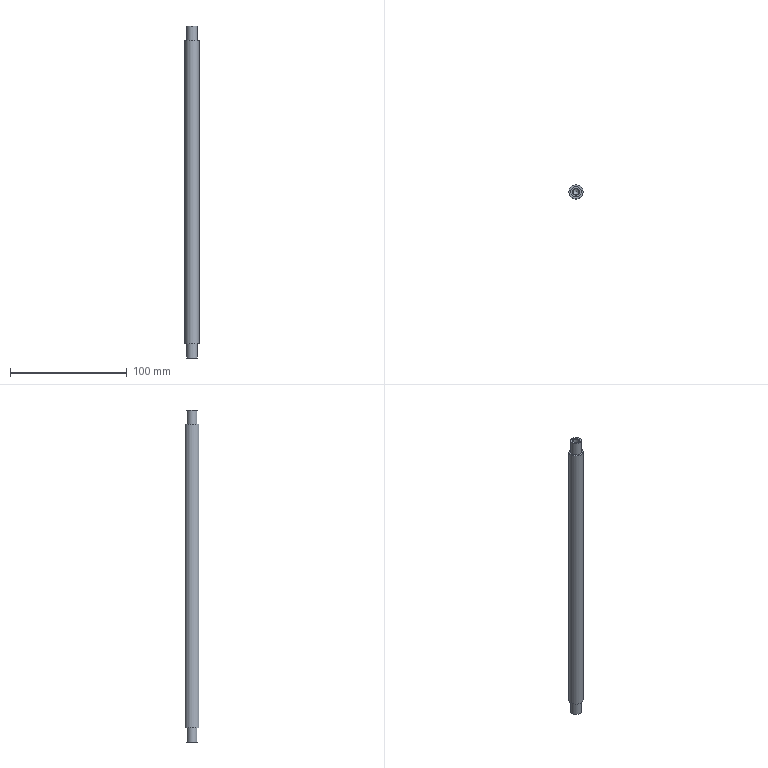Part | STEP file | YBQDJ-PD-13 | 1 solid | 13 faces | box 12 x 12 x 284 mm | volume 30280 mm3 | cylinder 5 | plane 4 | cone 4 | commonest cylinder face diameters 5 x2 9 x2 12 x1
STEP:
#1=CARTESIAN_POINT('',(0.,0.,0.));
#2=DIRECTION('',(0.,0.,1.));
#3=DIRECTION('',(1.,0.,0.));
#4=AXIS2_PLACEMENT_3D('',#1,#2,#3);
#5=CARTESIAN_POINT('',(-143.,400.,19.));
#6=VERTEX_POINT('',#5);
#7=CARTESIAN_POINT('',(-138.5,400.,19.));
#8=DIRECTION('',(0.,0.,-1.));
#9=DIRECTION('',(-1.,0.,0.));
#10=AXIS2_PLACEMENT_3D('',#7,#8,#9);
#11=CIRCLE('',#10,4.5);
#12=CARTESIAN_POINT('',(-108.5,415.,19.));
#13=DIRECTION('',(0.,0.,1.));
#14=DIRECTION('',(1.,0.,0.));
#15=AXIS2_PLACEMENT_3D('',#12,#13,#14);
#16=PLANE('',#15);
#17=CARTESIAN_POINT('',(-34.5,-15.));
#18=CARTESIAN_POINT('',(-34.5,-7.206));
#19=CARTESIAN_POINT('',(-27.75,-11.103));
#20=CARTESIAN_POINT('',(-21.,-15.));
#21=CARTESIAN_POINT('',(-27.75,-18.897));
#22=CARTESIAN_POINT('',(-34.5,-22.794));
#23=CARTESIAN_POINT('',(-34.5,-15.));
#24=(BOUNDED_CURVE()B_SPLINE_CURVE(2,(#17,#18,#19,#20,#21,#22,#23),.UNSPECIFIED.,.T.,.F.)B_SPLINE_CURVE_WITH_KNOTS((1,2,2,2,2,1),(-2.094,0.,2.094,4.189,6.283,8.378),.UNSPECIFIED.)CURVE()GEOMETRIC_REPRESENTATION_ITEM()RATIONAL_B_SPLINE_CURVE((1.,0.5,1.,0.5,1.,0.5,1.))REPRESENTATION_ITEM(''));
#25=(GEOMETRIC_REPRESENTATION_CONTEXT(2)PARAMETRIC_REPRESENTATION_CONTEXT()REPRESENTATION_CONTEXT('',''));
#26=DEFINITIONAL_REPRESENTATION('',(#24),#25);
#27=PCURVE('',#16,#26);
#28=CARTESIAN_POINT('',(-138.5,400.,7.));
#29=DIRECTION('',(0.,0.,1.));
#30=DIRECTION('',(1.,0.,0.));
#31=AXIS2_PLACEMENT_3D('',#28,#29,#30);
#32=CYLINDRICAL_SURFACE('',#31,4.5);
#33=CARTESIAN_POINT('',(9.425,12.));
#34=DIRECTION('',(-1.,0.));
#35=VECTOR('',#34,1.);
#36=LINE('',#33,#35);
#37=(GEOMETRIC_REPRESENTATION_CONTEXT(2)PARAMETRIC_REPRESENTATION_CONTEXT()REPRESENTATION_CONTEXT('',''));
#38=DEFINITIONAL_REPRESENTATION('',(#36),#37);
#39=PCURVE('',#32,#38);
#40=SURFACE_CURVE('',#11,(#27,#39),.PCURVE_S1.);
#41=EDGE_CURVE('',#6,#6,#40,.T.);
#42=ORIENTED_EDGE('',*,*,#41,.F.);
#43=EDGE_LOOP('',(#42));
#44=FACE_BOUND('',#43,.T.);
#45=CARTESIAN_POINT('',(-132.5,400.,19.));
#46=VERTEX_POINT('',#45);
#47=CARTESIAN_POINT('',(-138.5,400.,19.));
#48=DIRECTION('',(0.,0.,-1.));
#49=DIRECTION('',(1.,0.,0.));
#50=AXIS2_PLACEMENT_3D('',#47,#48,#49);
#51=CIRCLE('',#50,6.);
#52=CARTESIAN_POINT('',(-24.,-15.));
#53=CARTESIAN_POINT('',(-24.,-25.392));
#54=CARTESIAN_POINT('',(-33.,-20.196));
#55=CARTESIAN_POINT('',(-42.,-15.));
#56=CARTESIAN_POINT('',(-33.,-9.804));
#57=CARTESIAN_POINT('',(-24.,-4.608));
#58=CARTESIAN_POINT('',(-24.,-15.));
#59=(BOUNDED_CURVE()B_SPLINE_CURVE(2,(#52,#53,#54,#55,#56,#57,#58),.UNSPECIFIED.,.T.,.F.)B_SPLINE_CURVE_WITH_KNOTS((1,2,2,2,2,1),(-2.094,0.,2.094,4.189,6.283,8.378),.UNSPECIFIED.)CURVE()GEOMETRIC_REPRESENTATION_ITEM()RATIONAL_B_SPLINE_CURVE((1.,0.5,1.,0.5,1.,0.5,1.))REPRESENTATION_ITEM(''));
#60=(GEOMETRIC_REPRESENTATION_CONTEXT(2)PARAMETRIC_REPRESENTATION_CONTEXT()REPRESENTATION_CONTEXT('',''));
#61=DEFINITIONAL_REPRESENTATION('',(#59),#60);
#62=PCURVE('',#16,#61);
#63=CARTESIAN_POINT('',(-138.5,400.,-960.));
#64=DIRECTION('',(0.,0.,1.));
#65=DIRECTION('',(1.,0.,0.));
#66=AXIS2_PLACEMENT_3D('',#63,#64,#65);
#67=CYLINDRICAL_SURFACE('',#66,6.);
#68=CARTESIAN_POINT('',(6.283,979.));
#69=DIRECTION('',(-1.,0.));
#70=VECTOR('',#69,1.);
#71=LINE('',#68,#70);
#72=(GEOMETRIC_REPRESENTATION_CONTEXT(2)PARAMETRIC_REPRESENTATION_CONTEXT()REPRESENTATION_CONTEXT('',''));
#73=DEFINITIONAL_REPRESENTATION('',(#71),#72);
#74=PCURVE('',#67,#73);
#75=SURFACE_CURVE('',#51,(#62,#74),.PCURVE_S1.);
#76=EDGE_CURVE('',#46,#46,#75,.T.);
#77=ORIENTED_EDGE('',*,*,#76,.T.);
#78=EDGE_LOOP('',(#77));
#79=FACE_BOUND('',#78,.T.);
#80=ADVANCED_FACE('',(#44,#79),#16,.F.);
#81=CARTESIAN_POINT('',(-143.,400.,279.));
#82=VERTEX_POINT('',#81);
#83=CARTESIAN_POINT('',(-138.5,400.,279.));
#84=DIRECTION('',(0.,0.,-1.));
#85=DIRECTION('',(-1.,0.,0.));
#86=AXIS2_PLACEMENT_3D('',#83,#84,#85);
#87=CIRCLE('',#86,4.5);
#88=CARTESIAN_POINT('',(-134.5,400.,279.));
#89=DIRECTION('',(0.,0.,-1.));
#90=DIRECTION('',(-1.,0.,0.));
#91=AXIS2_PLACEMENT_3D('',#88,#89,#90);
#92=PLANE('',#91);
#93=CARTESIAN_POINT('',(4.,0.));
#94=DIRECTION('',(1.,0.));
#95=AXIS2_PLACEMENT_2D('',#93,#94);
#96=CIRCLE('',#95,4.5);
#97=(GEOMETRIC_REPRESENTATION_CONTEXT(2)PARAMETRIC_REPRESENTATION_CONTEXT()REPRESENTATION_CONTEXT('',''));
#98=DEFINITIONAL_REPRESENTATION('',(#96),#97);
#99=PCURVE('',#92,#98);
#100=CARTESIAN_POINT('',(-138.5,400.,291.));
#101=DIRECTION('',(0.,0.,-1.));
#102=DIRECTION('',(-1.,0.,0.));
#103=AXIS2_PLACEMENT_3D('',#100,#101,#102);
#104=CYLINDRICAL_SURFACE('',#103,4.5);
#105=CARTESIAN_POINT('',(0.,12.));
#106=DIRECTION('',(1.,0.));
#107=VECTOR('',#106,1.);
#108=LINE('',#105,#107);
#109=(GEOMETRIC_REPRESENTATION_CONTEXT(2)PARAMETRIC_REPRESENTATION_CONTEXT()REPRESENTATION_CONTEXT('',''));
#110=DEFINITIONAL_REPRESENTATION('',(#108),#109);
#111=PCURVE('',#104,#110);
#112=SURFACE_CURVE('',#87,(#99,#111),.PCURVE_S1.);
#113=EDGE_CURVE('',#82,#82,#112,.T.);
#114=ORIENTED_EDGE('',*,*,#113,.T.);
#115=EDGE_LOOP('',(#114));
#116=FACE_BOUND('',#115,.T.);
#117=CARTESIAN_POINT('',(-144.5,400.,279.));
#118=VERTEX_POINT('',#117);
#119=CARTESIAN_POINT('',(-132.5,400.,279.));
#120=VERTEX_POINT('',#119);
#121=CARTESIAN_POINT('',(-138.5,400.,279.));
#122=DIRECTION('',(0.,0.,-1.));
#123=DIRECTION('',(-1.,0.,0.));
#124=AXIS2_PLACEMENT_3D('',#121,#122,#123);
#125=CIRCLE('',#124,6.);
#126=CARTESIAN_POINT('',(4.,0.));
#127=DIRECTION('',(1.,0.));
#128=AXIS2_PLACEMENT_2D('',#126,#127);
#129=CIRCLE('',#128,6.);
#130=(GEOMETRIC_REPRESENTATION_CONTEXT(2)PARAMETRIC_REPRESENTATION_CONTEXT()REPRESENTATION_CONTEXT('',''));
#131=DEFINITIONAL_REPRESENTATION('',(#129),#130);
#132=PCURVE('',#92,#131);
#133=CARTESIAN_POINT('',(3.142,1239.));
#134=DIRECTION('',(-1.,0.));
#135=VECTOR('',#134,1.);
#136=LINE('',#133,#135);
#137=(GEOMETRIC_REPRESENTATION_CONTEXT(2)PARAMETRIC_REPRESENTATION_CONTEXT()REPRESENTATION_CONTEXT('',''));
#138=DEFINITIONAL_REPRESENTATION('',(#136),#137);
#139=PCURVE('',#67,#138);
#140=SURFACE_CURVE('',#125,(#132,#139),.PCURVE_S1.);
#141=EDGE_CURVE('',#118,#120,#140,.T.);
#142=ORIENTED_EDGE('',*,*,#141,.F.);
#143=CARTESIAN_POINT('',(-138.5,400.,279.));
#144=DIRECTION('',(0.,0.,-1.));
#145=DIRECTION('',(-1.,0.,0.));
#146=AXIS2_PLACEMENT_3D('',#143,#144,#145);
#147=CIRCLE('',#146,6.);
#148=CARTESIAN_POINT('',(4.,0.));
#149=DIRECTION('',(1.,0.));
#150=AXIS2_PLACEMENT_2D('',#148,#149);
#151=CIRCLE('',#150,6.);
#152=(GEOMETRIC_REPRESENTATION_CONTEXT(2)PARAMETRIC_REPRESENTATION_CONTEXT()REPRESENTATION_CONTEXT('',''));
#153=DEFINITIONAL_REPRESENTATION('',(#151),#152);
#154=PCURVE('',#92,#153);
#155=CARTESIAN_POINT('',(9.425,1239.));
#156=DIRECTION('',(-1.,0.));
#157=VECTOR('',#156,1.);
#158=LINE('',#155,#157);
#159=(GEOMETRIC_REPRESENTATION_CONTEXT(2)PARAMETRIC_REPRESENTATION_CONTEXT()REPRESENTATION_CONTEXT('',''));
#160=DEFINITIONAL_REPRESENTATION('',(#158),#159);
#161=PCURVE('',#67,#160);
#162=SURFACE_CURVE('',#147,(#154,#161),.PCURVE_S1.);
#163=EDGE_CURVE('',#120,#118,#162,.T.);
#164=ORIENTED_EDGE('',*,*,#163,.F.);
#165=EDGE_LOOP('',(#142,#164));
#166=FACE_BOUND('',#165,.T.);
#167=ADVANCED_FACE('',(#116,#166),#92,.F.);
#168=ORIENTED_EDGE('',*,*,#76,.F.);
#169=CARTESIAN_POINT('',(-132.5,400.,19.));
#170=CARTESIAN_POINT('',(-132.5,400.,279.));
#171=B_SPLINE_CURVE_WITH_KNOTS('',1,(#169,#170),.UNSPECIFIED.,.F.,.F.,(2,2),(979.,1239.),.PIECEWISE_BEZIER_KNOTS.);
#172=CARTESIAN_POINT('',(6.283,0.));
#173=DIRECTION('',(0.,1.));
#174=VECTOR('',#173,1.);
#175=LINE('',#172,#174);
#176=(GEOMETRIC_REPRESENTATION_CONTEXT(2)PARAMETRIC_REPRESENTATION_CONTEXT()REPRESENTATION_CONTEXT('',''));
#177=DEFINITIONAL_REPRESENTATION('',(#175),#176);
#178=PCURVE('',#67,#177);
#179=CARTESIAN_POINT('',(0.,0.));
#180=DIRECTION('',(0.,1.));
#181=VECTOR('',#180,1.);
#182=LINE('',#179,#181);
#183=(GEOMETRIC_REPRESENTATION_CONTEXT(2)PARAMETRIC_REPRESENTATION_CONTEXT()REPRESENTATION_CONTEXT('',''));
#184=DEFINITIONAL_REPRESENTATION('',(#182),#183);
#185=PCURVE('',#67,#184);
#186=SEAM_CURVE('',#171,(#178,#185),.PCURVE_S1.);
#187=EDGE_CURVE('',#46,#120,#186,.T.);
#188=ORIENTED_EDGE('',*,*,#187,.T.);
#189=ORIENTED_EDGE('',*,*,#163,.T.);
#190=ORIENTED_EDGE('',*,*,#141,.T.);
#191=ORIENTED_EDGE('',*,*,#187,.F.);
#192=EDGE_LOOP('',(#168,#188,#189,#190,#191));
#193=FACE_BOUND('',#192,.T.);
#194=ADVANCED_FACE('',(#193),#67,.T.);
#195=CARTESIAN_POINT('',(-143.,400.,291.));
#196=VERTEX_POINT('',#195);
#197=CARTESIAN_POINT('',(-138.5,400.,291.));
#198=DIRECTION('',(0.,0.,-1.));
#199=DIRECTION('',(-1.,0.,0.));
#200=AXIS2_PLACEMENT_3D('',#197,#198,#199);
#201=CIRCLE('',#200,4.5);
#202=CARTESIAN_POINT('',(0.,0.));
#203=DIRECTION('',(1.,0.));
#204=VECTOR('',#203,1.);
#205=LINE('',#202,#204);
#206=(GEOMETRIC_REPRESENTATION_CONTEXT(2)PARAMETRIC_REPRESENTATION_CONTEXT()REPRESENTATION_CONTEXT('',''));
#207=DEFINITIONAL_REPRESENTATION('',(#205),#206);
#208=PCURVE('',#104,#207);
#209=CARTESIAN_POINT('',(-138.5,400.,291.));
#210=DIRECTION('',(0.,0.,-1.));
#211=DIRECTION('',(-1.,0.,0.));
#212=AXIS2_PLACEMENT_3D('',#209,#210,#211);
#213=PLANE('',#212);
#214=CARTESIAN_POINT('',(0.,0.));
#215=DIRECTION('',(1.,0.));
#216=AXIS2_PLACEMENT_2D('',#214,#215);
#217=CIRCLE('',#216,4.5);
#218=(GEOMETRIC_REPRESENTATION_CONTEXT(2)PARAMETRIC_REPRESENTATION_CONTEXT()REPRESENTATION_CONTEXT('',''));
#219=DEFINITIONAL_REPRESENTATION('',(#217),#218);
#220=PCURVE('',#213,#219);
#221=SURFACE_CURVE('',#201,(#208,#220),.PCURVE_S1.);
#222=EDGE_CURVE('',#196,#196,#221,.T.);
#223=ORIENTED_EDGE('',*,*,#222,.T.);
#224=CARTESIAN_POINT('',(-143.,400.,291.));
#225=CARTESIAN_POINT('',(-143.,400.,279.));
#226=B_SPLINE_CURVE_WITH_KNOTS('',1,(#224,#225),.UNSPECIFIED.,.F.,.F.,(2,2),(0.,12.),.PIECEWISE_BEZIER_KNOTS.);
#227=CARTESIAN_POINT('',(6.283,0.));
#228=DIRECTION('',(0.,1.));
#229=VECTOR('',#228,1.);
#230=LINE('',#227,#229);
#231=(GEOMETRIC_REPRESENTATION_CONTEXT(2)PARAMETRIC_REPRESENTATION_CONTEXT()REPRESENTATION_CONTEXT('',''));
#232=DEFINITIONAL_REPRESENTATION('',(#230),#231);
#233=PCURVE('',#104,#232);
#234=CARTESIAN_POINT('',(0.,0.));
#235=DIRECTION('',(0.,1.));
#236=VECTOR('',#235,1.);
#237=LINE('',#234,#236);
#238=(GEOMETRIC_REPRESENTATION_CONTEXT(2)PARAMETRIC_REPRESENTATION_CONTEXT()REPRESENTATION_CONTEXT('',''));
#239=DEFINITIONAL_REPRESENTATION('',(#237),#238);
#240=PCURVE('',#104,#239);
#241=SEAM_CURVE('',#226,(#233,#240),.PCURVE_S1.);
#242=EDGE_CURVE('',#196,#82,#241,.T.);
#243=ORIENTED_EDGE('',*,*,#242,.T.);
#244=ORIENTED_EDGE('',*,*,#113,.F.);
#245=ORIENTED_EDGE('',*,*,#242,.F.);
#246=EDGE_LOOP('',(#223,#243,#244,#245));
#247=FACE_BOUND('',#246,.T.);
#248=ADVANCED_FACE('',(#247),#104,.T.);
#249=CARTESIAN_POINT('',(-141.5,400.,291.));
#250=VERTEX_POINT('',#249);
#251=CARTESIAN_POINT('',(-138.5,400.,291.));
#252=DIRECTION('',(0.,0.,-1.));
#253=DIRECTION('',(-1.,0.,0.));
#254=AXIS2_PLACEMENT_3D('',#251,#252,#253);
#255=CIRCLE('',#254,3.);
#256=CARTESIAN_POINT('',(0.,0.));
#257=DIRECTION('',(1.,0.));
#258=AXIS2_PLACEMENT_2D('',#256,#257);
#259=CIRCLE('',#258,3.);
#260=(GEOMETRIC_REPRESENTATION_CONTEXT(2)PARAMETRIC_REPRESENTATION_CONTEXT()REPRESENTATION_CONTEXT('',''));
#261=DEFINITIONAL_REPRESENTATION('',(#259),#260);
#262=PCURVE('',#213,#261);
#263=CARTESIAN_POINT('',(-138.5,400.,291.));
#264=DIRECTION('',(0.,0.,1.));
#265=DIRECTION('',(1.,0.,0.));
#266=AXIS2_PLACEMENT_3D('',#263,#264,#265);
#267=CONICAL_SURFACE('',#266,3.,0.7854);
#268=CARTESIAN_POINT('',(9.425,0.));
#269=DIRECTION('',(-1.,0.));
#270=VECTOR('',#269,1.);
#271=LINE('',#268,#270);
#272=(GEOMETRIC_REPRESENTATION_CONTEXT(2)PARAMETRIC_REPRESENTATION_CONTEXT()REPRESENTATION_CONTEXT('',''));
#273=DEFINITIONAL_REPRESENTATION('',(#271),#272);
#274=PCURVE('',#267,#273);
#275=SURFACE_CURVE('',#255,(#262,#274),.PCURVE_S1.);
#276=EDGE_CURVE('',#250,#250,#275,.T.);
#277=ORIENTED_EDGE('',*,*,#276,.T.);
#278=EDGE_LOOP('',(#277));
#279=FACE_BOUND('',#278,.T.);
#280=ORIENTED_EDGE('',*,*,#222,.F.);
#281=EDGE_LOOP('',(#280));
#282=FACE_BOUND('',#281,.T.);
#283=ADVANCED_FACE('',(#279,#282),#213,.F.);
#284=CARTESIAN_POINT('',(-136.,400.,279.));
#285=VERTEX_POINT('',#284);
#286=CARTESIAN_POINT('',(-141.,400.,279.));
#287=VERTEX_POINT('',#286);
#288=CARTESIAN_POINT('',(-138.5,400.,279.));
#289=DIRECTION('',(0.,0.,1.));
#290=DIRECTION('',(-1.,0.,0.));
#291=AXIS2_PLACEMENT_3D('',#288,#289,#290);
#292=CIRCLE('',#291,2.5);
#293=CARTESIAN_POINT('',(-138.5,400.,279.));
#294=DIRECTION('',(0.,0.,1.));
#295=DIRECTION('',(1.,0.,0.));
#296=AXIS2_PLACEMENT_3D('',#293,#294,#295);
#297=CONICAL_SURFACE('',#296,2.5,1.03);
#298=CARTESIAN_POINT('',(-3.142,0.));
#299=DIRECTION('',(1.,0.));
#300=VECTOR('',#299,1.);
#301=LINE('',#298,#300);
#302=(GEOMETRIC_REPRESENTATION_CONTEXT(2)PARAMETRIC_REPRESENTATION_CONTEXT()REPRESENTATION_CONTEXT('',''));
#303=DEFINITIONAL_REPRESENTATION('',(#301),#302);
#304=PCURVE('',#297,#303);
#305=CARTESIAN_POINT('',(-138.5,400.,291.));
#306=DIRECTION('',(0.,0.,-1.));
#307=DIRECTION('',(-1.,0.,0.));
#308=AXIS2_PLACEMENT_3D('',#305,#306,#307);
#309=CYLINDRICAL_SURFACE('',#308,2.5);
#310=CARTESIAN_POINT('',(6.283,12.));
#311=DIRECTION('',(-1.,0.));
#312=VECTOR('',#311,1.);
#313=LINE('',#310,#312);
#314=(GEOMETRIC_REPRESENTATION_CONTEXT(2)PARAMETRIC_REPRESENTATION_CONTEXT()REPRESENTATION_CONTEXT('',''));
#315=DEFINITIONAL_REPRESENTATION('',(#313),#314);
#316=PCURVE('',#309,#315);
#317=SURFACE_CURVE('',#292,(#304,#316),.PCURVE_S1.);
#318=EDGE_CURVE('',#285,#287,#317,.T.);
#319=ORIENTED_EDGE('',*,*,#318,.F.);
#320=CARTESIAN_POINT('',(-138.5,400.,277.498));
#321=VERTEX_POINT('',#320);
#322=CARTESIAN_POINT('',(-138.5,400.,277.498));
#323=CARTESIAN_POINT('',(-136.,400.,279.));
#324=B_SPLINE_CURVE_WITH_KNOTS('',1,(#322,#323),.UNSPECIFIED.,.F.,.F.,(2,2),(-2.917,0.),.PIECEWISE_BEZIER_KNOTS.);
#325=CARTESIAN_POINT('',(0.,0.));
#326=DIRECTION('',(0.,1.));
#327=VECTOR('',#326,1.);
#328=LINE('',#325,#327);
#329=(GEOMETRIC_REPRESENTATION_CONTEXT(2)PARAMETRIC_REPRESENTATION_CONTEXT()REPRESENTATION_CONTEXT('',''));
#330=DEFINITIONAL_REPRESENTATION('',(#328),#329);
#331=PCURVE('',#297,#330);
#332=CARTESIAN_POINT('',(6.283,0.));
#333=DIRECTION('',(0.,1.));
#334=VECTOR('',#333,1.);
#335=LINE('',#332,#334);
#336=(GEOMETRIC_REPRESENTATION_CONTEXT(2)PARAMETRIC_REPRESENTATION_CONTEXT()REPRESENTATION_CONTEXT('',''));
#337=DEFINITIONAL_REPRESENTATION('',(#335),#336);
#338=PCURVE('',#297,#337);
#339=SEAM_CURVE('',#324,(#331,#338),.PCURVE_S1.);
#340=EDGE_CURVE('',#321,#285,#339,.T.);
#341=ORIENTED_EDGE('',*,*,#340,.F.);
#342=ORIENTED_EDGE('',*,*,#340,.T.);
#343=CARTESIAN_POINT('',(-138.5,400.,279.));
#344=DIRECTION('',(0.,0.,1.));
#345=DIRECTION('',(-1.,0.,0.));
#346=AXIS2_PLACEMENT_3D('',#343,#344,#345);
#347=CIRCLE('',#346,2.5);
#348=CARTESIAN_POINT('',(3.142,0.));
#349=DIRECTION('',(1.,0.));
#350=VECTOR('',#349,1.);
#351=LINE('',#348,#350);
#352=(GEOMETRIC_REPRESENTATION_CONTEXT(2)PARAMETRIC_REPRESENTATION_CONTEXT()REPRESENTATION_CONTEXT('',''));
#353=DEFINITIONAL_REPRESENTATION('',(#351),#352);
#354=PCURVE('',#297,#353);
#355=CARTESIAN_POINT('',(6.283,12.));
#356=DIRECTION('',(-1.,0.));
#357=VECTOR('',#356,1.);
#358=LINE('',#355,#357);
#359=(GEOMETRIC_REPRESENTATION_CONTEXT(2)PARAMETRIC_REPRESENTATION_CONTEXT()REPRESENTATION_CONTEXT('',''));
#360=DEFINITIONAL_REPRESENTATION('',(#358),#359);
#361=PCURVE('',#309,#360);
#362=SURFACE_CURVE('',#347,(#354,#361),.PCURVE_S1.);
#363=EDGE_CURVE('',#287,#285,#362,.T.);
#364=ORIENTED_EDGE('',*,*,#363,.F.);
#365=EDGE_LOOP('',(#319,#341,#342,#364));
#366=FACE_BOUND('',#365,.F.);
#367=ADVANCED_FACE('',(#366),#297,.F.);
#368=CARTESIAN_POINT('',(-141.,400.,290.5));
#369=VERTEX_POINT('',#368);
#370=CARTESIAN_POINT('',(-138.5,400.,290.5));
#371=DIRECTION('',(0.,0.,1.));
#372=DIRECTION('',(-1.,0.,0.));
#373=AXIS2_PLACEMENT_3D('',#370,#371,#372);
#374=CIRCLE('',#373,2.5);
#375=CARTESIAN_POINT('',(6.283,0.5));
#376=DIRECTION('',(-1.,0.));
#377=VECTOR('',#376,1.);
#378=LINE('',#375,#377);
#379=(GEOMETRIC_REPRESENTATION_CONTEXT(2)PARAMETRIC_REPRESENTATION_CONTEXT()REPRESENTATION_CONTEXT('',''));
#380=DEFINITIONAL_REPRESENTATION('',(#378),#379);
#381=PCURVE('',#309,#380);
#382=CARTESIAN_POINT('',(3.142,-0.5));
#383=DIRECTION('',(1.,0.));
#384=VECTOR('',#383,1.);
#385=LINE('',#382,#384);
#386=(GEOMETRIC_REPRESENTATION_CONTEXT(2)PARAMETRIC_REPRESENTATION_CONTEXT()REPRESENTATION_CONTEXT('',''));
#387=DEFINITIONAL_REPRESENTATION('',(#385),#386);
#388=PCURVE('',#267,#387);
#389=SURFACE_CURVE('',#374,(#381,#388),.PCURVE_S1.);
#390=EDGE_CURVE('',#369,#369,#389,.T.);
#391=ORIENTED_EDGE('',*,*,#390,.F.);
#392=CARTESIAN_POINT('',(-141.,400.,290.5));
#393=CARTESIAN_POINT('',(-141.,400.,279.));
#394=B_SPLINE_CURVE_WITH_KNOTS('',1,(#392,#393),.UNSPECIFIED.,.F.,.F.,(2,2),(0.5,12.),.PIECEWISE_BEZIER_KNOTS.);
#395=CARTESIAN_POINT('',(6.283,0.));
#396=DIRECTION('',(0.,1.));
#397=VECTOR('',#396,1.);
#398=LINE('',#395,#397);
#399=(GEOMETRIC_REPRESENTATION_CONTEXT(2)PARAMETRIC_REPRESENTATION_CONTEXT()REPRESENTATION_CONTEXT('',''));
#400=DEFINITIONAL_REPRESENTATION('',(#398),#399);
#401=PCURVE('',#309,#400);
#402=CARTESIAN_POINT('',(0.,0.));
#403=DIRECTION('',(0.,1.));
#404=VECTOR('',#403,1.);
#405=LINE('',#402,#404);
#406=(GEOMETRIC_REPRESENTATION_CONTEXT(2)PARAMETRIC_REPRESENTATION_CONTEXT()REPRESENTATION_CONTEXT('',''));
#407=DEFINITIONAL_REPRESENTATION('',(#405),#406);
#408=PCURVE('',#309,#407);
#409=SEAM_CURVE('',#394,(#401,#408),.PCURVE_S1.);
#410=EDGE_CURVE('',#369,#287,#409,.T.);
#411=ORIENTED_EDGE('',*,*,#410,.T.);
#412=ORIENTED_EDGE('',*,*,#363,.T.);
#413=ORIENTED_EDGE('',*,*,#318,.T.);
#414=ORIENTED_EDGE('',*,*,#410,.F.);
#415=EDGE_LOOP('',(#391,#411,#412,#413,#414));
#416=FACE_BOUND('',#415,.F.);
#417=ADVANCED_FACE('',(#416),#309,.F.);
#418=ORIENTED_EDGE('',*,*,#390,.T.);
#419=CARTESIAN_POINT('',(-141.,400.,290.5));
#420=CARTESIAN_POINT('',(-141.5,400.,291.));
#421=B_SPLINE_CURVE_WITH_KNOTS('',1,(#419,#420),.UNSPECIFIED.,.F.,.F.,(2,2),(-0.7071,0.),.PIECEWISE_BEZIER_KNOTS.);
#422=CARTESIAN_POINT('',(9.425,0.));
#423=DIRECTION('',(0.,1.));
#424=VECTOR('',#423,1.);
#425=LINE('',#422,#424);
#426=(GEOMETRIC_REPRESENTATION_CONTEXT(2)PARAMETRIC_REPRESENTATION_CONTEXT()REPRESENTATION_CONTEXT('',''));
#427=DEFINITIONAL_REPRESENTATION('',(#425),#426);
#428=PCURVE('',#267,#427);
#429=CARTESIAN_POINT('',(3.142,0.));
#430=DIRECTION('',(0.,1.));
#431=VECTOR('',#430,1.);
#432=LINE('',#429,#431);
#433=(GEOMETRIC_REPRESENTATION_CONTEXT(2)PARAMETRIC_REPRESENTATION_CONTEXT()REPRESENTATION_CONTEXT('',''));
#434=DEFINITIONAL_REPRESENTATION('',(#432),#433);
#435=PCURVE('',#267,#434);
#436=SEAM_CURVE('',#421,(#428,#435),.PCURVE_S1.);
#437=EDGE_CURVE('',#369,#250,#436,.T.);
#438=ORIENTED_EDGE('',*,*,#437,.T.);
#439=ORIENTED_EDGE('',*,*,#276,.T.);
#440=ORIENTED_EDGE('',*,*,#437,.F.);
#441=EDGE_LOOP('',(#418,#438,#439,#440));
#442=FACE_BOUND('',#441,.F.);
#443=ADVANCED_FACE('',(#442),#267,.F.);
#444=CARTESIAN_POINT('',(-143.,400.,7.));
#445=VERTEX_POINT('',#444);
#446=CARTESIAN_POINT('',(-138.5,400.,7.));
#447=DIRECTION('',(0.,0.,-1.));
#448=DIRECTION('',(-1.,0.,0.));
#449=AXIS2_PLACEMENT_3D('',#446,#447,#448);
#450=CIRCLE('',#449,4.5);
#451=CARTESIAN_POINT('',(9.425,0.));
#452=DIRECTION('',(-1.,0.));
#453=VECTOR('',#452,1.);
#454=LINE('',#451,#453);
#455=(GEOMETRIC_REPRESENTATION_CONTEXT(2)PARAMETRIC_REPRESENTATION_CONTEXT()REPRESENTATION_CONTEXT('',''));
#456=DEFINITIONAL_REPRESENTATION('',(#454),#455);
#457=PCURVE('',#32,#456);
#458=CARTESIAN_POINT('',(-138.5,400.,7.));
#459=DIRECTION('',(0.,0.,-1.));
#460=DIRECTION('',(-1.,0.,0.));
#461=AXIS2_PLACEMENT_3D('',#458,#459,#460);
#462=PLANE('',#461);
#463=CARTESIAN_POINT('',(0.,0.));
#464=DIRECTION('',(1.,0.));
#465=AXIS2_PLACEMENT_2D('',#463,#464);
#466=CIRCLE('',#465,4.5);
#467=(GEOMETRIC_REPRESENTATION_CONTEXT(2)PARAMETRIC_REPRESENTATION_CONTEXT()REPRESENTATION_CONTEXT('',''));
#468=DEFINITIONAL_REPRESENTATION('',(#466),#467);
#469=PCURVE('',#462,#468);
#470=SURFACE_CURVE('',#450,(#457,#469),.PCURVE_S1.);
#471=EDGE_CURVE('',#445,#445,#470,.T.);
#472=ORIENTED_EDGE('',*,*,#471,.F.);
#473=CARTESIAN_POINT('',(-143.,400.,7.));
#474=CARTESIAN_POINT('',(-143.,400.,19.));
#475=B_SPLINE_CURVE_WITH_KNOTS('',1,(#473,#474),.UNSPECIFIED.,.F.,.F.,(2,2),(0.,12.),.PIECEWISE_BEZIER_KNOTS.);
#476=CARTESIAN_POINT('',(9.425,0.));
#477=DIRECTION('',(0.,1.));
#478=VECTOR('',#477,1.);
#479=LINE('',#476,#478);
#480=(GEOMETRIC_REPRESENTATION_CONTEXT(2)PARAMETRIC_REPRESENTATION_CONTEXT()REPRESENTATION_CONTEXT('',''));
#481=DEFINITIONAL_REPRESENTATION('',(#479),#480);
#482=PCURVE('',#32,#481);
#483=CARTESIAN_POINT('',(3.142,0.));
#484=DIRECTION('',(0.,1.));
#485=VECTOR('',#484,1.);
#486=LINE('',#483,#485);
#487=(GEOMETRIC_REPRESENTATION_CONTEXT(2)PARAMETRIC_REPRESENTATION_CONTEXT()REPRESENTATION_CONTEXT('',''));
#488=DEFINITIONAL_REPRESENTATION('',(#486),#487);
#489=PCURVE('',#32,#488);
#490=SEAM_CURVE('',#475,(#482,#489),.PCURVE_S1.);
#491=EDGE_CURVE('',#445,#6,#490,.T.);
#492=ORIENTED_EDGE('',*,*,#491,.T.);
#493=ORIENTED_EDGE('',*,*,#41,.T.);
#494=ORIENTED_EDGE('',*,*,#491,.F.);
#495=EDGE_LOOP('',(#472,#492,#493,#494));
#496=FACE_BOUND('',#495,.T.);
#497=ADVANCED_FACE('',(#496),#32,.T.);
#498=CARTESIAN_POINT('',(-141.5,400.,7.));
#499=VERTEX_POINT('',#498);
#500=CARTESIAN_POINT('',(-138.5,400.,7.));
#501=DIRECTION('',(0.,0.,1.));
#502=DIRECTION('',(-1.,0.,0.));
#503=AXIS2_PLACEMENT_3D('',#500,#501,#502);
#504=CIRCLE('',#503,3.);
#505=CARTESIAN_POINT('',(3.,0.));
#506=CARTESIAN_POINT('',(3.,-5.196));
#507=CARTESIAN_POINT('',(-1.5,-2.598));
#508=CARTESIAN_POINT('',(-6.,0.));
#509=CARTESIAN_POINT('',(-1.5,2.598));
#510=CARTESIAN_POINT('',(3.,5.196));
#511=CARTESIAN_POINT('',(3.,0.));
#512=(BOUNDED_CURVE()B_SPLINE_CURVE(2,(#505,#506,#507,#508,#509,#510,#511),.UNSPECIFIED.,.T.,.F.)B_SPLINE_CURVE_WITH_KNOTS((1,2,2,2,2,1),(-2.094,0.,2.094,4.189,6.283,8.378),.UNSPECIFIED.)CURVE()GEOMETRIC_REPRESENTATION_ITEM()RATIONAL_B_SPLINE_CURVE((1.,0.5,1.,0.5,1.,0.5,1.))REPRESENTATION_ITEM(''));
#513=(GEOMETRIC_REPRESENTATION_CONTEXT(2)PARAMETRIC_REPRESENTATION_CONTEXT()REPRESENTATION_CONTEXT('',''));
#514=DEFINITIONAL_REPRESENTATION('',(#512),#513);
#515=PCURVE('',#462,#514);
#516=CARTESIAN_POINT('',(-138.5,400.,7.));
#517=DIRECTION('',(0.,0.,-1.));
#518=DIRECTION('',(-1.,0.,0.));
#519=AXIS2_PLACEMENT_3D('',#516,#517,#518);
#520=CONICAL_SURFACE('',#519,3.,0.7854);
#521=CARTESIAN_POINT('',(6.283,0.));
#522=DIRECTION('',(-1.,0.));
#523=VECTOR('',#522,1.);
#524=LINE('',#521,#523);
#525=(GEOMETRIC_REPRESENTATION_CONTEXT(2)PARAMETRIC_REPRESENTATION_CONTEXT()REPRESENTATION_CONTEXT('',''));
#526=DEFINITIONAL_REPRESENTATION('',(#524),#525);
#527=PCURVE('',#520,#526);
#528=SURFACE_CURVE('',#504,(#515,#527),.PCURVE_S1.);
#529=EDGE_CURVE('',#499,#499,#528,.T.);
#530=ORIENTED_EDGE('',*,*,#529,.T.);
#531=EDGE_LOOP('',(#530));
#532=FACE_BOUND('',#531,.T.);
#533=ORIENTED_EDGE('',*,*,#471,.T.);
#534=EDGE_LOOP('',(#533));
#535=FACE_BOUND('',#534,.T.);
#536=ADVANCED_FACE('',(#532,#535),#462,.T.);
#537=CARTESIAN_POINT('',(-141.,400.,27.));
#538=VERTEX_POINT('',#537);
#539=CARTESIAN_POINT('',(-136.,400.,27.));
#540=VERTEX_POINT('',#539);
#541=CARTESIAN_POINT('',(-138.5,400.,27.));
#542=DIRECTION('',(0.,0.,-1.));
#543=DIRECTION('',(1.,0.,0.));
#544=AXIS2_PLACEMENT_3D('',#541,#542,#543);
#545=CIRCLE('',#544,2.5);
#546=CARTESIAN_POINT('',(-138.5,400.,27.));
#547=DIRECTION('',(0.,0.,-1.));
#548=DIRECTION('',(-1.,0.,0.));
#549=AXIS2_PLACEMENT_3D('',#546,#547,#548);
#550=CONICAL_SURFACE('',#549,2.5,1.03);
#551=CARTESIAN_POINT('',(-3.142,0.));
#552=DIRECTION('',(1.,0.));
#553=VECTOR('',#552,1.);
#554=LINE('',#551,#553);
#555=(GEOMETRIC_REPRESENTATION_CONTEXT(2)PARAMETRIC_REPRESENTATION_CONTEXT()REPRESENTATION_CONTEXT('',''));
#556=DEFINITIONAL_REPRESENTATION('',(#554),#555);
#557=PCURVE('',#550,#556);
#558=CARTESIAN_POINT('',(-138.5,400.,7.));
#559=DIRECTION('',(0.,0.,1.));
#560=DIRECTION('',(1.,0.,0.));
#561=AXIS2_PLACEMENT_3D('',#558,#559,#560);
#562=CYLINDRICAL_SURFACE('',#561,2.5);
#563=CARTESIAN_POINT('',(12.566,20.));
#564=DIRECTION('',(-1.,0.));
#565=VECTOR('',#564,1.);
#566=LINE('',#563,#565);
#567=(GEOMETRIC_REPRESENTATION_CONTEXT(2)PARAMETRIC_REPRESENTATION_CONTEXT()REPRESENTATION_CONTEXT('',''));
#568=DEFINITIONAL_REPRESENTATION('',(#566),#567);
#569=PCURVE('',#562,#568);
#570=SURFACE_CURVE('',#545,(#557,#569),.PCURVE_S1.);
#571=EDGE_CURVE('',#538,#540,#570,.T.);
#572=ORIENTED_EDGE('',*,*,#571,.F.);
#573=CARTESIAN_POINT('',(-138.5,400.,28.502));
#574=VERTEX_POINT('',#573);
#575=CARTESIAN_POINT('',(-138.5,400.,28.502));
#576=CARTESIAN_POINT('',(-141.,400.,27.));
#577=B_SPLINE_CURVE_WITH_KNOTS('',1,(#575,#576),.UNSPECIFIED.,.F.,.F.,(2,2),(-2.917,0.),.PIECEWISE_BEZIER_KNOTS.);
#578=CARTESIAN_POINT('',(0.,0.));
#579=DIRECTION('',(0.,1.));
#580=VECTOR('',#579,1.);
#581=LINE('',#578,#580);
#582=(GEOMETRIC_REPRESENTATION_CONTEXT(2)PARAMETRIC_REPRESENTATION_CONTEXT()REPRESENTATION_CONTEXT('',''));
#583=DEFINITIONAL_REPRESENTATION('',(#581),#582);
#584=PCURVE('',#550,#583);
#585=CARTESIAN_POINT('',(6.283,0.));
#586=DIRECTION('',(0.,1.));
#587=VECTOR('',#586,1.);
#588=LINE('',#585,#587);
#589=(GEOMETRIC_REPRESENTATION_CONTEXT(2)PARAMETRIC_REPRESENTATION_CONTEXT()REPRESENTATION_CONTEXT('',''));
#590=DEFINITIONAL_REPRESENTATION('',(#588),#589);
#591=PCURVE('',#550,#590);
#592=SEAM_CURVE('',#577,(#584,#591),.PCURVE_S1.);
#593=EDGE_CURVE('',#574,#538,#592,.T.);
#594=ORIENTED_EDGE('',*,*,#593,.F.);
#595=ORIENTED_EDGE('',*,*,#593,.T.);
#596=CARTESIAN_POINT('',(-138.5,400.,27.));
#597=DIRECTION('',(0.,0.,-1.));
#598=DIRECTION('',(1.,0.,0.));
#599=AXIS2_PLACEMENT_3D('',#596,#597,#598);
#600=CIRCLE('',#599,2.5);
#601=CARTESIAN_POINT('',(3.142,0.));
#602=DIRECTION('',(1.,0.));
#603=VECTOR('',#602,1.);
#604=LINE('',#601,#603);
#605=(GEOMETRIC_REPRESENTATION_CONTEXT(2)PARAMETRIC_REPRESENTATION_CONTEXT()REPRESENTATION_CONTEXT('',''));
#606=DEFINITIONAL_REPRESENTATION('',(#604),#605);
#607=PCURVE('',#550,#606);
#608=CARTESIAN_POINT('',(6.283,20.));
#609=DIRECTION('',(-1.,0.));
#610=VECTOR('',#609,1.);
#611=LINE('',#608,#610);
#612=(GEOMETRIC_REPRESENTATION_CONTEXT(2)PARAMETRIC_REPRESENTATION_CONTEXT()REPRESENTATION_CONTEXT('',''));
#613=DEFINITIONAL_REPRESENTATION('',(#611),#612);
#614=PCURVE('',#562,#613);
#615=SURFACE_CURVE('',#600,(#607,#614),.PCURVE_S1.);
#616=EDGE_CURVE('',#540,#538,#615,.T.);
#617=ORIENTED_EDGE('',*,*,#616,.F.);
#618=EDGE_LOOP('',(#572,#594,#595,#617));
#619=FACE_BOUND('',#618,.F.);
#620=ADVANCED_FACE('',(#619),#550,.F.);
#621=CARTESIAN_POINT('',(-141.,400.,7.5));
#622=VERTEX_POINT('',#621);
#623=CARTESIAN_POINT('',(-138.5,400.,7.5));
#624=DIRECTION('',(0.,0.,-1.));
#625=DIRECTION('',(-1.,0.,0.));
#626=AXIS2_PLACEMENT_3D('',#623,#624,#625);
#627=CIRCLE('',#626,2.5);
#628=CARTESIAN_POINT('',(9.425,0.5));
#629=DIRECTION('',(-1.,0.));
#630=VECTOR('',#629,1.);
#631=LINE('',#628,#630);
#632=(GEOMETRIC_REPRESENTATION_CONTEXT(2)PARAMETRIC_REPRESENTATION_CONTEXT()REPRESENTATION_CONTEXT('',''));
#633=DEFINITIONAL_REPRESENTATION('',(#631),#632);
#634=PCURVE('',#562,#633);
#635=CARTESIAN_POINT('',(0.,-0.5));
#636=DIRECTION('',(1.,0.));
#637=VECTOR('',#636,1.);
#638=LINE('',#635,#637);
#639=(GEOMETRIC_REPRESENTATION_CONTEXT(2)PARAMETRIC_REPRESENTATION_CONTEXT()REPRESENTATION_CONTEXT('',''));
#640=DEFINITIONAL_REPRESENTATION('',(#638),#639);
#641=PCURVE('',#520,#640);
#642=SURFACE_CURVE('',#627,(#634,#641),.PCURVE_S1.);
#643=EDGE_CURVE('',#622,#622,#642,.T.);
#644=ORIENTED_EDGE('',*,*,#643,.F.);
#645=CARTESIAN_POINT('',(-141.,400.,7.5));
#646=CARTESIAN_POINT('',(-141.,400.,27.));
#647=B_SPLINE_CURVE_WITH_KNOTS('',1,(#645,#646),.UNSPECIFIED.,.F.,.F.,(2,2),(0.5,20.),.PIECEWISE_BEZIER_KNOTS.);
#648=CARTESIAN_POINT('',(9.425,0.));
#649=DIRECTION('',(0.,1.));
#650=VECTOR('',#649,1.);
#651=LINE('',#648,#650);
#652=(GEOMETRIC_REPRESENTATION_CONTEXT(2)PARAMETRIC_REPRESENTATION_CONTEXT()REPRESENTATION_CONTEXT('',''));
#653=DEFINITIONAL_REPRESENTATION('',(#651),#652);
#654=PCURVE('',#562,#653);
#655=CARTESIAN_POINT('',(3.142,0.));
#656=DIRECTION('',(0.,1.));
#657=VECTOR('',#656,1.);
#658=LINE('',#655,#657);
#659=(GEOMETRIC_REPRESENTATION_CONTEXT(2)PARAMETRIC_REPRESENTATION_CONTEXT()REPRESENTATION_CONTEXT('',''));
#660=DEFINITIONAL_REPRESENTATION('',(#658),#659);
#661=PCURVE('',#562,#660);
#662=SEAM_CURVE('',#647,(#654,#661),.PCURVE_S1.);
#663=EDGE_CURVE('',#622,#538,#662,.T.);
#664=ORIENTED_EDGE('',*,*,#663,.T.);
#665=ORIENTED_EDGE('',*,*,#571,.T.);
#666=ORIENTED_EDGE('',*,*,#616,.T.);
#667=ORIENTED_EDGE('',*,*,#663,.F.);
#668=EDGE_LOOP('',(#644,#664,#665,#666,#667));
#669=FACE_BOUND('',#668,.F.);
#670=ADVANCED_FACE('',(#669),#562,.F.);
#671=ORIENTED_EDGE('',*,*,#643,.T.);
#672=CARTESIAN_POINT('',(-141.,400.,7.5));
#673=CARTESIAN_POINT('',(-141.5,400.,7.));
#674=B_SPLINE_CURVE_WITH_KNOTS('',1,(#672,#673),.UNSPECIFIED.,.F.,.F.,(2,2),(-0.7071,0.),.PIECEWISE_BEZIER_KNOTS.);
#675=CARTESIAN_POINT('',(6.283,0.));
#676=DIRECTION('',(0.,1.));
#677=VECTOR('',#676,1.);
#678=LINE('',#675,#677);
#679=(GEOMETRIC_REPRESENTATION_CONTEXT(2)PARAMETRIC_REPRESENTATION_CONTEXT()REPRESENTATION_CONTEXT('',''));
#680=DEFINITIONAL_REPRESENTATION('',(#678),#679);
#681=PCURVE('',#520,#680);
#682=CARTESIAN_POINT('',(0.,0.));
#683=DIRECTION('',(0.,1.));
#684=VECTOR('',#683,1.);
#685=LINE('',#682,#684);
#686=(GEOMETRIC_REPRESENTATION_CONTEXT(2)PARAMETRIC_REPRESENTATION_CONTEXT()REPRESENTATION_CONTEXT('',''));
#687=DEFINITIONAL_REPRESENTATION('',(#685),#686);
#688=PCURVE('',#520,#687);
#689=SEAM_CURVE('',#674,(#681,#688),.PCURVE_S1.);
#690=EDGE_CURVE('',#622,#499,#689,.T.);
#691=ORIENTED_EDGE('',*,*,#690,.T.);
#692=ORIENTED_EDGE('',*,*,#529,.T.);
#693=ORIENTED_EDGE('',*,*,#690,.F.);
#694=EDGE_LOOP('',(#671,#691,#692,#693));
#695=FACE_BOUND('',#694,.F.);
#696=ADVANCED_FACE('',(#695),#520,.F.);
#697=CLOSED_SHELL('',(#80,#167,#194,#248,#283,#367,#417,#443,#497,#536,#620,#670,#696));
#698=MANIFOLD_SOLID_BREP('',#697);
#699=(LENGTH_UNIT()NAMED_UNIT(*)SI_UNIT(.MILLI.,.METRE.));
#700=UNCERTAINTY_MEASURE_WITH_UNIT(LENGTH_MEASURE(0.00001),#699,'','');
#701=(NAMED_UNIT(*)PLANE_ANGLE_UNIT()SI_UNIT($,.RADIAN.));
#702=(NAMED_UNIT(*)SI_UNIT($,.STERADIAN.)SOLID_ANGLE_UNIT());
#703=(GEOMETRIC_REPRESENTATION_CONTEXT(3)GLOBAL_UNCERTAINTY_ASSIGNED_CONTEXT((#700))GLOBAL_UNIT_ASSIGNED_CONTEXT((#699,#701,#702))REPRESENTATION_CONTEXT('',''));
#704=ADVANCED_BREP_SHAPE_REPRESENTATION('',(#4,#698),#703);